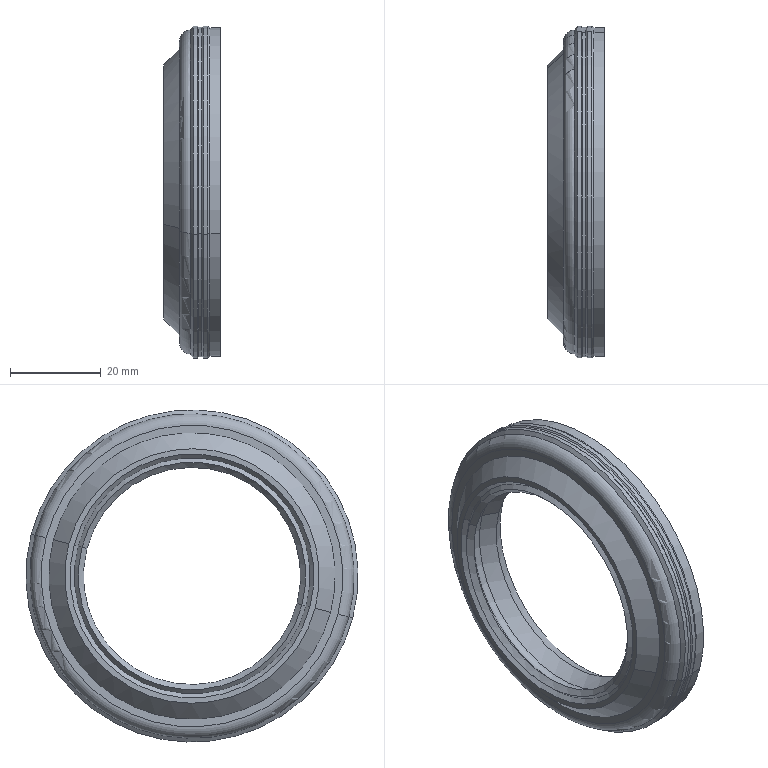Part | NX | features BREP 1 | 1 solid | 57 faces | box 12.5 x 73.025 x 73.025 mm | volume 15033 mm3 | cone 26 | torus 14 | cylinder 12 | plane 5 | commonest cylinder face diameters 53.4 x4 73.025 x4 72.34 x2 72.479 x2
STEP:
#1=CARTESIAN_POINT('',(-614.47,-25.827,-6.773));
#2=VERTEX_POINT('',#1);
#3=CARTESIAN_POINT('',(-614.47,25.827,6.773));
#4=VERTEX_POINT('',#3);
#5=CARTESIAN_POINT('',(-614.47,0.,0.));
#6=DIRECTION('',(-1.,0.,0.));
#7=DIRECTION('',(0.,-0.9673,-0.2537));
#8=AXIS2_PLACEMENT_3D('',#5,#6,#7);
#9=CIRCLE('',#8,26.7);
#10=EDGE_CURVE('',#2,#4,#9,.T.);
#11=ORIENTED_EDGE('',*,*,#10,.T.);
#12=CARTESIAN_POINT('',(-617.27,25.827,6.773));
#13=VERTEX_POINT('',#12);
#14=CARTESIAN_POINT('',(-615.87,25.827,6.773));
#15=DIRECTION('',(0.,-0.2537,0.9673));
#16=DIRECTION('',(0.,-0.9673,-0.2537));
#17=AXIS2_PLACEMENT_3D('',#14,#15,#16);
#18=CIRCLE('',#17,1.4);
#19=EDGE_CURVE('',#13,#4,#18,.F.);
#20=ORIENTED_EDGE('',*,*,#19,.F.);
#21=CARTESIAN_POINT('',(-617.27,-25.827,-6.773));
#22=VERTEX_POINT('',#21);
#23=CARTESIAN_POINT('',(-617.27,0.,0.));
#24=DIRECTION('',(1.,0.,0.));
#25=DIRECTION('',(0.,0.9673,0.2537));
#26=AXIS2_PLACEMENT_3D('',#23,#24,#25);
#27=CIRCLE('',#26,26.7);
#28=EDGE_CURVE('',#13,#22,#27,.T.);
#29=ORIENTED_EDGE('',*,*,#28,.T.);
#30=CARTESIAN_POINT('',(-615.87,-25.827,-6.773));
#31=DIRECTION('',(0.,0.2537,-0.9673));
#32=DIRECTION('',(0.,0.9673,0.2537));
#33=AXIS2_PLACEMENT_3D('',#30,#31,#32);
#34=CIRCLE('',#33,1.4);
#35=EDGE_CURVE('',#22,#2,#34,.F.);
#36=ORIENTED_EDGE('',*,*,#35,.T.);
#37=EDGE_LOOP('',(#11,#20,#29,#36));
#38=FACE_BOUND('',#37,.T.);
#39=CARTESIAN_POINT('',(-615.87,0.,0.));
#40=DIRECTION('',(-1.,0.,0.));
#41=DIRECTION('',(0.,0.9673,0.2537));
#42=AXIS2_PLACEMENT_3D('',#39,#40,#41);
#43=TOROIDAL_SURFACE('',#42,26.7,1.4);
#44=ADVANCED_FACE('',(#38),#43,.T.);
#45=CARTESIAN_POINT('',(-616.197,35.054,9.192));
#46=VERTEX_POINT('',#45);
#47=CARTESIAN_POINT('',(-616.197,-35.054,-9.192));
#48=VERTEX_POINT('',#47);
#49=CARTESIAN_POINT('',(-616.197,0.,0.));
#50=DIRECTION('',(1.,0.,0.));
#51=DIRECTION('',(0.,0.9673,0.2537));
#52=AXIS2_PLACEMENT_3D('',#49,#50,#51);
#53=CIRCLE('',#52,36.24);
#54=EDGE_CURVE('',#46,#48,#53,.T.);
#55=ORIENTED_EDGE('',*,*,#54,.T.);
#56=CARTESIAN_POINT('',(-615.494,-35.054,-9.192));
#57=VERTEX_POINT('',#56);
#58=CARTESIAN_POINT('',(-613.72,-35.054,-9.192));
#59=DIRECTION('',(1.,0.,0.));
#60=VECTOR('',#59,1000.);
#61=LINE('',#58,#60);
#62=EDGE_CURVE('',#48,#57,#61,.T.);
#63=ORIENTED_EDGE('',*,*,#62,.T.);
#64=CARTESIAN_POINT('',(-615.494,35.054,9.192));
#65=VERTEX_POINT('',#64);
#66=CARTESIAN_POINT('',(-615.494,0.,0.));
#67=DIRECTION('',(1.,0.,0.));
#68=DIRECTION('',(0.,0.9673,0.2537));
#69=AXIS2_PLACEMENT_3D('',#66,#67,#68);
#70=CIRCLE('',#69,36.24);
#71=EDGE_CURVE('',#65,#57,#70,.T.);
#72=ORIENTED_EDGE('',*,*,#71,.F.);
#73=CARTESIAN_POINT('',(-613.72,35.054,9.192));
#74=DIRECTION('',(1.,0.,0.));
#75=VECTOR('',#74,1000.);
#76=LINE('',#73,#75);
#77=EDGE_CURVE('',#46,#65,#76,.T.);
#78=ORIENTED_EDGE('',*,*,#77,.F.);
#79=EDGE_LOOP('',(#55,#63,#72,#78));
#80=FACE_BOUND('',#79,.T.);
#81=CARTESIAN_POINT('',(-613.72,0.,0.));
#82=DIRECTION('',(1.,0.,0.));
#83=DIRECTION('',(0.,-0.9673,-0.2537));
#84=AXIS2_PLACEMENT_3D('',#81,#82,#83);
#85=CYLINDRICAL_SURFACE('',#84,36.24);
#86=ADVANCED_FACE('',(#80),#85,.T.);
#87=ORIENTED_EDGE('',*,*,#71,.T.);
#88=CARTESIAN_POINT('',(-615.221,-35.318,-9.262));
#89=VERTEX_POINT('',#88);
#90=CARTESIAN_POINT('',(-615.221,-35.318,-9.262));
#91=DIRECTION('',(0.7071,-0.684,-0.1794));
#92=VECTOR('',#91,1000.);
#93=LINE('',#90,#92);
#94=EDGE_CURVE('',#57,#89,#93,.T.);
#95=ORIENTED_EDGE('',*,*,#94,.T.);
#96=CARTESIAN_POINT('',(-615.221,35.318,9.262));
#97=VERTEX_POINT('',#96);
#98=CARTESIAN_POINT('',(-615.221,0.,0.));
#99=DIRECTION('',(1.,0.,0.));
#100=DIRECTION('',(0.,0.9673,0.2537));
#101=AXIS2_PLACEMENT_3D('',#98,#99,#100);
#102=CIRCLE('',#101,36.513);
#103=EDGE_CURVE('',#97,#89,#102,.T.);
#104=ORIENTED_EDGE('',*,*,#103,.F.);
#105=CARTESIAN_POINT('',(-615.221,35.318,9.262));
#106=DIRECTION('',(0.7071,0.684,0.1794));
#107=VECTOR('',#106,1000.);
#108=LINE('',#105,#107);
#109=EDGE_CURVE('',#65,#97,#108,.T.);
#110=ORIENTED_EDGE('',*,*,#109,.F.);
#111=EDGE_LOOP('',(#87,#95,#104,#110));
#112=FACE_BOUND('',#111,.T.);
#113=CARTESIAN_POINT('',(-615.221,0.,0.));
#114=DIRECTION('',(1.,0.,0.));
#115=DIRECTION('',(0.,-0.9673,-0.2537));
#116=AXIS2_PLACEMENT_3D('',#113,#114,#115);
#117=CONICAL_SURFACE('',#116,36.513,0.7854);
#118=ADVANCED_FACE('',(#112),#117,.T.);
#119=ORIENTED_EDGE('',*,*,#103,.T.);
#120=CARTESIAN_POINT('',(-614.28,-35.318,-9.262));
#121=VERTEX_POINT('',#120);
#122=CARTESIAN_POINT('',(-613.72,-35.318,-9.262));
#123=DIRECTION('',(1.,0.,0.));
#124=VECTOR('',#123,1000.);
#125=LINE('',#122,#124);
#126=EDGE_CURVE('',#89,#121,#125,.T.);
#127=ORIENTED_EDGE('',*,*,#126,.T.);
#128=CARTESIAN_POINT('',(-614.28,35.318,9.262));
#129=VERTEX_POINT('',#128);
#130=CARTESIAN_POINT('',(-614.28,0.,0.));
#131=DIRECTION('',(1.,0.,0.));
#132=DIRECTION('',(0.,0.9673,0.2537));
#133=AXIS2_PLACEMENT_3D('',#130,#131,#132);
#134=CIRCLE('',#133,36.513);
#135=EDGE_CURVE('',#129,#121,#134,.T.);
#136=ORIENTED_EDGE('',*,*,#135,.F.);
#137=CARTESIAN_POINT('',(-613.72,35.318,9.262));
#138=DIRECTION('',(1.,0.,0.));
#139=VECTOR('',#138,1000.);
#140=LINE('',#137,#139);
#141=EDGE_CURVE('',#97,#129,#140,.T.);
#142=ORIENTED_EDGE('',*,*,#141,.F.);
#143=EDGE_LOOP('',(#119,#127,#136,#142));
#144=FACE_BOUND('',#143,.T.);
#145=CARTESIAN_POINT('',(-613.72,0.,0.));
#146=DIRECTION('',(1.,0.,0.));
#147=DIRECTION('',(0.,-0.9673,-0.2537));
#148=AXIS2_PLACEMENT_3D('',#145,#146,#147);
#149=CYLINDRICAL_SURFACE('',#148,36.513);
#150=ADVANCED_FACE('',(#144),#149,.T.);
#151=CARTESIAN_POINT('',(-613.72,-34.987,-9.175));
#152=VERTEX_POINT('',#151);
#153=CARTESIAN_POINT('',(-613.72,34.987,9.175));
#154=VERTEX_POINT('',#153);
#155=CARTESIAN_POINT('',(-613.72,0.,0.));
#156=DIRECTION('',(-1.,0.,0.));
#157=DIRECTION('',(0.,-0.9673,-0.2537));
#158=AXIS2_PLACEMENT_3D('',#155,#156,#157);
#159=CIRCLE('',#158,36.17);
#160=EDGE_CURVE('',#152,#154,#159,.T.);
#161=ORIENTED_EDGE('',*,*,#160,.T.);
#162=CARTESIAN_POINT('',(-613.72,34.987,9.175));
#163=DIRECTION('',(-0.8529,0.5049,0.1324));
#164=VECTOR('',#163,1000.);
#165=LINE('',#162,#164);
#166=EDGE_CURVE('',#129,#154,#165,.F.);
#167=ORIENTED_EDGE('',*,*,#166,.F.);
#168=ORIENTED_EDGE('',*,*,#135,.T.);
#169=CARTESIAN_POINT('',(-613.72,-34.987,-9.175));
#170=DIRECTION('',(-0.8529,-0.5049,-0.1324));
#171=VECTOR('',#170,1000.);
#172=LINE('',#169,#171);
#173=EDGE_CURVE('',#121,#152,#172,.F.);
#174=ORIENTED_EDGE('',*,*,#173,.T.);
#175=EDGE_LOOP('',(#161,#167,#168,#174));
#176=FACE_BOUND('',#175,.T.);
#177=CARTESIAN_POINT('',(-613.72,0.,0.));
#178=DIRECTION('',(-1.,0.,0.));
#179=DIRECTION('',(0.,0.9673,0.2537));
#180=AXIS2_PLACEMENT_3D('',#177,#178,#179);
#181=CONICAL_SURFACE('',#180,36.17,0.5492);
#182=ADVANCED_FACE('',(#176),#181,.T.);
#183=CARTESIAN_POINT('',(-618.051,34.481,9.042));
#184=VERTEX_POINT('',#183);
#185=CARTESIAN_POINT('',(-618.051,-34.481,-9.042));
#186=VERTEX_POINT('',#185);
#187=CARTESIAN_POINT('',(-618.051,0.,0.));
#188=DIRECTION('',(1.,0.,0.));
#189=DIRECTION('',(0.,0.9673,0.2537));
#190=AXIS2_PLACEMENT_3D('',#187,#188,#189);
#191=CIRCLE('',#190,35.647);
#192=EDGE_CURVE('',#184,#186,#191,.T.);
#193=ORIENTED_EDGE('',*,*,#192,.T.);
#194=CARTESIAN_POINT('',(-617.43,-35.318,-9.262));
#195=VERTEX_POINT('',#194);
#196=CARTESIAN_POINT('',(-617.43,-35.318,-9.262));
#197=DIRECTION('',(0.5827,-0.7861,-0.2061));
#198=VECTOR('',#197,1000.);
#199=LINE('',#196,#198);
#200=EDGE_CURVE('',#186,#195,#199,.T.);
#201=ORIENTED_EDGE('',*,*,#200,.T.);
#202=CARTESIAN_POINT('',(-617.43,35.318,9.262));
#203=VERTEX_POINT('',#202);
#204=CARTESIAN_POINT('',(-617.43,0.,0.));
#205=DIRECTION('',(1.,0.,0.));
#206=DIRECTION('',(0.,0.9673,0.2537));
#207=AXIS2_PLACEMENT_3D('',#204,#205,#206);
#208=CIRCLE('',#207,36.513);
#209=EDGE_CURVE('',#203,#195,#208,.T.);
#210=ORIENTED_EDGE('',*,*,#209,.F.);
#211=CARTESIAN_POINT('',(-617.43,35.318,9.262));
#212=DIRECTION('',(0.5827,0.7861,0.2061));
#213=VECTOR('',#212,1000.);
#214=LINE('',#211,#213);
#215=EDGE_CURVE('',#184,#203,#214,.T.);
#216=ORIENTED_EDGE('',*,*,#215,.F.);
#217=EDGE_LOOP('',(#193,#201,#210,#216));
#218=FACE_BOUND('',#217,.T.);
#219=CARTESIAN_POINT('',(-617.43,0.,0.));
#220=DIRECTION('',(1.,0.,0.));
#221=DIRECTION('',(0.,-0.9673,-0.2537));
#222=AXIS2_PLACEMENT_3D('',#219,#220,#221);
#223=CONICAL_SURFACE('',#222,36.513,0.9488);
#224=ADVANCED_FACE('',(#218),#223,.T.);
#225=ORIENTED_EDGE('',*,*,#209,.T.);
#226=CARTESIAN_POINT('',(-616.47,-35.318,-9.262));
#227=VERTEX_POINT('',#226);
#228=CARTESIAN_POINT('',(-613.72,-35.318,-9.262));
#229=DIRECTION('',(1.,0.,0.));
#230=VECTOR('',#229,1000.);
#231=LINE('',#228,#230);
#232=EDGE_CURVE('',#195,#227,#231,.T.);
#233=ORIENTED_EDGE('',*,*,#232,.T.);
#234=CARTESIAN_POINT('',(-616.47,35.318,9.262));
#235=VERTEX_POINT('',#234);
#236=CARTESIAN_POINT('',(-616.47,0.,0.));
#237=DIRECTION('',(1.,0.,0.));
#238=DIRECTION('',(0.,0.9673,0.2537));
#239=AXIS2_PLACEMENT_3D('',#236,#237,#238);
#240=CIRCLE('',#239,36.513);
#241=EDGE_CURVE('',#235,#227,#240,.T.);
#242=ORIENTED_EDGE('',*,*,#241,.F.);
#243=CARTESIAN_POINT('',(-613.72,35.318,9.262));
#244=DIRECTION('',(1.,0.,0.));
#245=VECTOR('',#244,1000.);
#246=LINE('',#243,#245);
#247=EDGE_CURVE('',#203,#235,#246,.T.);
#248=ORIENTED_EDGE('',*,*,#247,.F.);
#249=EDGE_LOOP('',(#225,#233,#242,#248));
#250=FACE_BOUND('',#249,.T.);
#251=CARTESIAN_POINT('',(-613.72,0.,0.));
#252=DIRECTION('',(1.,0.,0.));
#253=DIRECTION('',(0.,-0.9673,-0.2537));
#254=AXIS2_PLACEMENT_3D('',#251,#252,#253);
#255=CYLINDRICAL_SURFACE('',#254,36.513);
#256=ADVANCED_FACE('',(#250),#255,.T.);
#257=ORIENTED_EDGE('',*,*,#54,.F.);
#258=CARTESIAN_POINT('',(-616.197,35.054,9.192));
#259=DIRECTION('',(-0.7071,0.684,0.1794));
#260=VECTOR('',#259,1000.);
#261=LINE('',#258,#260);
#262=EDGE_CURVE('',#235,#46,#261,.F.);
#263=ORIENTED_EDGE('',*,*,#262,.F.);
#264=ORIENTED_EDGE('',*,*,#241,.T.);
#265=CARTESIAN_POINT('',(-616.197,-35.054,-9.192));
#266=DIRECTION('',(-0.7071,-0.684,-0.1794));
#267=VECTOR('',#266,1000.);
#268=LINE('',#265,#267);
#269=EDGE_CURVE('',#227,#48,#268,.F.);
#270=ORIENTED_EDGE('',*,*,#269,.T.);
#271=EDGE_LOOP('',(#257,#263,#264,#270));
#272=FACE_BOUND('',#271,.T.);
#273=CARTESIAN_POINT('',(-616.197,0.,0.));
#274=DIRECTION('',(-1.,0.,0.));
#275=DIRECTION('',(0.,0.9673,0.2537));
#276=AXIS2_PLACEMENT_3D('',#273,#274,#275);
#277=CONICAL_SURFACE('',#276,36.24,0.7854);
#278=ADVANCED_FACE('',(#272),#277,.T.);
#279=CARTESIAN_POINT('',(-611.42,-34.987,-9.175));
#280=VERTEX_POINT('',#279);
#281=CARTESIAN_POINT('',(-611.42,34.987,9.175));
#282=VERTEX_POINT('',#281);
#283=CARTESIAN_POINT('',(-611.42,0.,0.));
#284=DIRECTION('',(-1.,0.,0.));
#285=DIRECTION('',(0.,-0.9673,-0.2537));
#286=AXIS2_PLACEMENT_3D('',#283,#284,#285);
#287=CIRCLE('',#286,36.17);
#288=EDGE_CURVE('',#280,#282,#287,.T.);
#289=ORIENTED_EDGE('',*,*,#288,.T.);
#290=CARTESIAN_POINT('',(-623.62,34.987,9.175));
#291=DIRECTION('',(-1.,0.,0.));
#292=VECTOR('',#291,1000.);
#293=LINE('',#290,#292);
#294=EDGE_CURVE('',#154,#282,#293,.F.);
#295=ORIENTED_EDGE('',*,*,#294,.F.);
#296=ORIENTED_EDGE('',*,*,#160,.F.);
#297=CARTESIAN_POINT('',(-623.62,-34.987,-9.175));
#298=DIRECTION('',(-1.,0.,0.));
#299=VECTOR('',#298,1000.);
#300=LINE('',#297,#299);
#301=EDGE_CURVE('',#152,#280,#300,.F.);
#302=ORIENTED_EDGE('',*,*,#301,.T.);
#303=EDGE_LOOP('',(#289,#295,#296,#302));
#304=FACE_BOUND('',#303,.T.);
#305=CARTESIAN_POINT('',(-623.62,0.,0.));
#306=DIRECTION('',(-1.,0.,0.));
#307=DIRECTION('',(0.,0.9673,0.2537));
#308=AXIS2_PLACEMENT_3D('',#305,#306,#307);
#309=CYLINDRICAL_SURFACE('',#308,36.17);
#310=ADVANCED_FACE('',(#304),#309,.T.);
#311=ORIENTED_EDGE('',*,*,#192,.F.);
#312=CARTESIAN_POINT('',(-620.42,32.066,8.409));
#313=VERTEX_POINT('',#312);
#314=CARTESIAN_POINT('',(-617.92,32.066,8.409));
#315=DIRECTION('',(0.,-0.2537,0.9673));
#316=DIRECTION('',(0.,-0.9673,-0.2537));
#317=AXIS2_PLACEMENT_3D('',#314,#315,#316);
#318=CIRCLE('',#317,2.5);
#319=EDGE_CURVE('',#313,#184,#318,.F.);
#320=ORIENTED_EDGE('',*,*,#319,.F.);
#321=CARTESIAN_POINT('',(-620.42,-32.066,-8.409));
#322=VERTEX_POINT('',#321);
#323=CARTESIAN_POINT('',(-620.42,0.,0.));
#324=DIRECTION('',(-1.,0.,0.));
#325=DIRECTION('',(0.,-0.9673,-0.2537));
#326=AXIS2_PLACEMENT_3D('',#323,#324,#325);
#327=CIRCLE('',#326,33.15);
#328=EDGE_CURVE('',#322,#313,#327,.T.);
#329=ORIENTED_EDGE('',*,*,#328,.F.);
#330=CARTESIAN_POINT('',(-617.92,-32.066,-8.409));
#331=DIRECTION('',(0.,0.2537,-0.9673));
#332=DIRECTION('',(0.,0.9673,0.2537));
#333=AXIS2_PLACEMENT_3D('',#330,#331,#332);
#334=CIRCLE('',#333,2.5);
#335=EDGE_CURVE('',#322,#186,#334,.F.);
#336=ORIENTED_EDGE('',*,*,#335,.T.);
#337=EDGE_LOOP('',(#311,#320,#329,#336));
#338=FACE_BOUND('',#337,.T.);
#339=CARTESIAN_POINT('',(-617.92,0.,0.));
#340=DIRECTION('',(-1.,0.,0.));
#341=DIRECTION('',(0.,0.9673,0.2537));
#342=AXIS2_PLACEMENT_3D('',#339,#340,#341);
#343=TOROIDAL_SURFACE('',#342,33.15,2.5);
#344=ADVANCED_FACE('',(#338),#343,.T.);
#345=CARTESIAN_POINT('',(-615.87,23.094,6.056));
#346=VERTEX_POINT('',#345);
#347=CARTESIAN_POINT('',(-615.87,-23.094,-6.056));
#348=VERTEX_POINT('',#347);
#349=CARTESIAN_POINT('',(-615.87,0.,0.));
#350=DIRECTION('',(-1.,0.,0.));
#351=DIRECTION('',(0.,-0.9673,-0.2537));
#352=AXIS2_PLACEMENT_3D('',#349,#350,#351);
#353=CIRCLE('',#352,23.875);
#354=EDGE_CURVE('',#346,#348,#353,.T.);
#355=ORIENTED_EDGE('',*,*,#354,.F.);
#356=CARTESIAN_POINT('',(-619.575,24.542,6.436));
#357=VERTEX_POINT('',#356);
#358=CARTESIAN_POINT('',(-619.575,24.542,6.436));
#359=DIRECTION('',(-0.9272,0.3624,0.09502));
#360=VECTOR('',#359,1000.);
#361=LINE('',#358,#360);
#362=EDGE_CURVE('',#357,#346,#361,.F.);
#363=ORIENTED_EDGE('',*,*,#362,.F.);
#364=CARTESIAN_POINT('',(-619.575,-24.542,-6.436));
#365=VERTEX_POINT('',#364);
#366=CARTESIAN_POINT('',(-619.575,0.,0.));
#367=DIRECTION('',(-1.,0.,0.));
#368=DIRECTION('',(0.,-0.9673,-0.2537));
#369=AXIS2_PLACEMENT_3D('',#366,#367,#368);
#370=CIRCLE('',#369,25.372);
#371=EDGE_CURVE('',#357,#365,#370,.T.);
#372=ORIENTED_EDGE('',*,*,#371,.T.);
#373=CARTESIAN_POINT('',(-619.575,-24.542,-6.436));
#374=DIRECTION('',(-0.9272,-0.3624,-0.09502));
#375=VECTOR('',#374,1000.);
#376=LINE('',#373,#375);
#377=EDGE_CURVE('',#365,#348,#376,.F.);
#378=ORIENTED_EDGE('',*,*,#377,.T.);
#379=EDGE_LOOP('',(#355,#363,#372,#378));
#380=FACE_BOUND('',#379,.T.);
#381=CARTESIAN_POINT('',(-619.575,0.,0.));
#382=DIRECTION('',(-1.,0.,0.));
#383=DIRECTION('',(0.,0.9673,0.2537));
#384=AXIS2_PLACEMENT_3D('',#381,#382,#383);
#385=CONICAL_SURFACE('',#384,25.372,0.384);
#386=ADVANCED_FACE('',(#380),#385,.F.);
#387=ORIENTED_EDGE('',*,*,#354,.T.);
#388=CARTESIAN_POINT('',(-613.07,-24.666,-6.468));
#389=VERTEX_POINT('',#388);
#390=CARTESIAN_POINT('',(-615.87,-23.094,-6.056));
#391=DIRECTION('',(0.8649,-0.4855,-0.1273));
#392=VECTOR('',#391,1000.);
#393=LINE('',#390,#392);
#394=EDGE_CURVE('',#348,#389,#393,.T.);
#395=ORIENTED_EDGE('',*,*,#394,.T.);
#396=CARTESIAN_POINT('',(-613.07,24.666,6.468));
#397=VERTEX_POINT('',#396);
#398=CARTESIAN_POINT('',(-613.07,0.,0.));
#399=DIRECTION('',(-1.,0.,0.));
#400=DIRECTION('',(0.,-0.9673,-0.2537));
#401=AXIS2_PLACEMENT_3D('',#398,#399,#400);
#402=CIRCLE('',#401,25.5);
#403=EDGE_CURVE('',#397,#389,#402,.T.);
#404=ORIENTED_EDGE('',*,*,#403,.F.);
#405=CARTESIAN_POINT('',(-615.87,23.094,6.056));
#406=DIRECTION('',(0.8649,0.4855,0.1273));
#407=VECTOR('',#406,1000.);
#408=LINE('',#405,#407);
#409=EDGE_CURVE('',#346,#397,#408,.T.);
#410=ORIENTED_EDGE('',*,*,#409,.F.);
#411=EDGE_LOOP('',(#387,#395,#404,#410));
#412=FACE_BOUND('',#411,.T.);
#413=CARTESIAN_POINT('',(-615.87,0.,0.));
#414=DIRECTION('',(1.,0.,0.));
#415=DIRECTION('',(0.,-0.9673,-0.2537));
#416=AXIS2_PLACEMENT_3D('',#413,#414,#415);
#417=CONICAL_SURFACE('',#416,23.875,0.5259);
#418=ADVANCED_FACE('',(#412),#417,.F.);
#419=CARTESIAN_POINT('',(-613.07,-25.827,-6.773));
#420=VERTEX_POINT('',#419);
#421=CARTESIAN_POINT('',(-613.07,25.827,6.773));
#422=VERTEX_POINT('',#421);
#423=CARTESIAN_POINT('',(-613.07,0.,0.));
#424=DIRECTION('',(-1.,0.,0.));
#425=DIRECTION('',(0.,-0.9673,-0.2537));
#426=AXIS2_PLACEMENT_3D('',#423,#424,#425);
#427=CIRCLE('',#426,26.7);
#428=EDGE_CURVE('',#420,#422,#427,.T.);
#429=ORIENTED_EDGE('',*,*,#428,.T.);
#430=CARTESIAN_POINT('',(-623.92,25.827,6.773));
#431=DIRECTION('',(-1.,0.,0.));
#432=VECTOR('',#431,1000.);
#433=LINE('',#430,#432);
#434=EDGE_CURVE('',#4,#422,#433,.F.);
#435=ORIENTED_EDGE('',*,*,#434,.F.);
#436=ORIENTED_EDGE('',*,*,#10,.F.);
#437=CARTESIAN_POINT('',(-623.92,-25.827,-6.773));
#438=DIRECTION('',(-1.,0.,0.));
#439=VECTOR('',#438,1000.);
#440=LINE('',#437,#439);
#441=EDGE_CURVE('',#2,#420,#440,.F.);
#442=ORIENTED_EDGE('',*,*,#441,.T.);
#443=EDGE_LOOP('',(#429,#435,#436,#442));
#444=FACE_BOUND('',#443,.T.);
#445=CARTESIAN_POINT('',(-623.92,0.,0.));
#446=DIRECTION('',(-1.,0.,0.));
#447=DIRECTION('',(0.,0.9673,0.2537));
#448=AXIS2_PLACEMENT_3D('',#445,#446,#447);
#449=CYLINDRICAL_SURFACE('',#448,26.7);
#450=ADVANCED_FACE('',(#444),#449,.T.);
#451=ORIENTED_EDGE('',*,*,#28,.F.);
#452=CARTESIAN_POINT('',(-618.787,25.827,6.773));
#453=VERTEX_POINT('',#452);
#454=CARTESIAN_POINT('',(-623.92,25.827,6.773));
#455=DIRECTION('',(-1.,0.,0.));
#456=VECTOR('',#455,1000.);
#457=LINE('',#454,#456);
#458=EDGE_CURVE('',#453,#13,#457,.F.);
#459=ORIENTED_EDGE('',*,*,#458,.F.);
#460=CARTESIAN_POINT('',(-618.787,-25.827,-6.773));
#461=VERTEX_POINT('',#460);
#462=CARTESIAN_POINT('',(-618.787,0.,0.));
#463=DIRECTION('',(-1.,0.,0.));
#464=DIRECTION('',(0.,-0.9673,-0.2537));
#465=AXIS2_PLACEMENT_3D('',#462,#463,#464);
#466=CIRCLE('',#465,26.7);
#467=EDGE_CURVE('',#461,#453,#466,.T.);
#468=ORIENTED_EDGE('',*,*,#467,.F.);
#469=CARTESIAN_POINT('',(-623.92,-25.827,-6.773));
#470=DIRECTION('',(-1.,0.,0.));
#471=VECTOR('',#470,1000.);
#472=LINE('',#469,#471);
#473=EDGE_CURVE('',#461,#22,#472,.F.);
#474=ORIENTED_EDGE('',*,*,#473,.T.);
#475=EDGE_LOOP('',(#451,#459,#468,#474));
#476=FACE_BOUND('',#475,.T.);
#477=CARTESIAN_POINT('',(-623.92,0.,0.));
#478=DIRECTION('',(-1.,0.,0.));
#479=DIRECTION('',(0.,0.9673,0.2537));
#480=AXIS2_PLACEMENT_3D('',#477,#478,#479);
#481=CYLINDRICAL_SURFACE('',#480,26.7);
#482=ADVANCED_FACE('',(#476),#481,.T.);
#483=CARTESIAN_POINT('',(-619.07,26.487,6.946));
#484=VERTEX_POINT('',#483);
#485=CARTESIAN_POINT('',(-619.07,-26.487,-6.946));
#486=VERTEX_POINT('',#485);
#487=CARTESIAN_POINT('',(-619.07,0.,0.));
#488=DIRECTION('',(-1.,0.,0.));
#489=DIRECTION('',(0.,-0.9673,-0.2537));
#490=AXIS2_PLACEMENT_3D('',#487,#488,#489);
#491=CIRCLE('',#490,27.383);
#492=EDGE_CURVE('',#484,#486,#491,.T.);
#493=ORIENTED_EDGE('',*,*,#492,.F.);
#494=CARTESIAN_POINT('',(-618.787,26.214,6.874));
#495=DIRECTION('',(0.,-0.2537,0.9673));
#496=DIRECTION('',(0.,-0.9673,-0.2537));
#497=AXIS2_PLACEMENT_3D('',#494,#495,#496);
#498=CIRCLE('',#497,0.4);
#499=EDGE_CURVE('',#453,#484,#498,.F.);
#500=ORIENTED_EDGE('',*,*,#499,.F.);
#501=CARTESIAN_POINT('',(-618.787,0.,0.));
#502=DIRECTION('',(-1.,0.,0.));
#503=DIRECTION('',(0.,-0.9673,-0.2537));
#504=AXIS2_PLACEMENT_3D('',#501,#502,#503);
#505=CIRCLE('',#504,26.7);
#506=EDGE_CURVE('',#453,#461,#505,.T.);
#507=ORIENTED_EDGE('',*,*,#506,.T.);
#508=CARTESIAN_POINT('',(-618.787,-26.214,-6.874));
#509=DIRECTION('',(0.,0.2537,-0.9673));
#510=DIRECTION('',(0.,0.9673,0.2537));
#511=AXIS2_PLACEMENT_3D('',#508,#509,#510);
#512=CIRCLE('',#511,0.4);
#513=EDGE_CURVE('',#461,#486,#512,.F.);
#514=ORIENTED_EDGE('',*,*,#513,.T.);
#515=EDGE_LOOP('',(#493,#500,#507,#514));
#516=FACE_BOUND('',#515,.T.);
#517=CARTESIAN_POINT('',(-618.787,0.,0.));
#518=DIRECTION('',(-1.,0.,0.));
#519=DIRECTION('',(0.,0.9673,0.2537));
#520=AXIS2_PLACEMENT_3D('',#517,#518,#519);
#521=TOROIDAL_SURFACE('',#520,27.1,0.4);
#522=ADVANCED_FACE('',(#516),#521,.F.);
#523=ORIENTED_EDGE('',*,*,#492,.T.);
#524=CARTESIAN_POINT('',(-618.233,-27.297,-7.158));
#525=VERTEX_POINT('',#524);
#526=CARTESIAN_POINT('',(-619.07,-26.487,-6.946));
#527=DIRECTION('',(0.7071,-0.684,-0.1794));
#528=VECTOR('',#527,1000.);
#529=LINE('',#526,#528);
#530=EDGE_CURVE('',#486,#525,#529,.T.);
#531=ORIENTED_EDGE('',*,*,#530,.T.);
#532=CARTESIAN_POINT('',(-618.233,27.297,7.158));
#533=VERTEX_POINT('',#532);
#534=CARTESIAN_POINT('',(-618.233,0.,0.));
#535=DIRECTION('',(-1.,0.,0.));
#536=DIRECTION('',(0.,-0.9673,-0.2537));
#537=AXIS2_PLACEMENT_3D('',#534,#535,#536);
#538=CIRCLE('',#537,28.22);
#539=EDGE_CURVE('',#533,#525,#538,.T.);
#540=ORIENTED_EDGE('',*,*,#539,.F.);
#541=CARTESIAN_POINT('',(-619.07,26.487,6.946));
#542=DIRECTION('',(0.7071,0.684,0.1794));
#543=VECTOR('',#542,1000.);
#544=LINE('',#541,#543);
#545=EDGE_CURVE('',#484,#533,#544,.T.);
#546=ORIENTED_EDGE('',*,*,#545,.F.);
#547=EDGE_LOOP('',(#523,#531,#540,#546));
#548=FACE_BOUND('',#547,.T.);
#549=CARTESIAN_POINT('',(-619.07,0.,0.));
#550=DIRECTION('',(1.,0.,0.));
#551=DIRECTION('',(0.,-0.9673,-0.2537));
#552=AXIS2_PLACEMENT_3D('',#549,#550,#551);
#553=CONICAL_SURFACE('',#552,27.383,0.7854);
#554=ADVANCED_FACE('',(#548),#553,.F.);
#555=CARTESIAN_POINT('',(-618.233,0.,0.));
#556=DIRECTION('',(-1.,0.,0.));
#557=DIRECTION('',(0.,-0.9673,-0.2537));
#558=AXIS2_PLACEMENT_3D('',#555,#556,#557);
#559=CIRCLE('',#558,28.22);
#560=EDGE_CURVE('',#525,#533,#559,.T.);
#561=ORIENTED_EDGE('',*,*,#560,.T.);
#562=CARTESIAN_POINT('',(-617.12,29.896,7.84));
#563=VERTEX_POINT('',#562);
#564=CARTESIAN_POINT('',(-620.92,29.896,7.84));
#565=DIRECTION('',(0.,-0.2537,0.9673));
#566=DIRECTION('',(0.,-0.9673,-0.2537));
#567=AXIS2_PLACEMENT_3D('',#564,#565,#566);
#568=CIRCLE('',#567,3.8);
#569=EDGE_CURVE('',#563,#533,#568,.F.);
#570=ORIENTED_EDGE('',*,*,#569,.F.);
#571=CARTESIAN_POINT('',(-617.12,-29.896,-7.84));
#572=VERTEX_POINT('',#571);
#573=CARTESIAN_POINT('',(-617.12,0.,0.));
#574=DIRECTION('',(-1.,0.,0.));
#575=DIRECTION('',(0.,-0.9673,-0.2537));
#576=AXIS2_PLACEMENT_3D('',#573,#574,#575);
#577=CIRCLE('',#576,30.907);
#578=EDGE_CURVE('',#572,#563,#577,.T.);
#579=ORIENTED_EDGE('',*,*,#578,.F.);
#580=CARTESIAN_POINT('',(-620.92,-29.896,-7.84));
#581=DIRECTION('',(0.,0.2537,-0.9673));
#582=DIRECTION('',(0.,0.9673,0.2537));
#583=AXIS2_PLACEMENT_3D('',#580,#581,#582);
#584=CIRCLE('',#583,3.8);
#585=EDGE_CURVE('',#572,#525,#584,.F.);
#586=ORIENTED_EDGE('',*,*,#585,.T.);
#587=EDGE_LOOP('',(#561,#570,#579,#586));
#588=FACE_BOUND('',#587,.T.);
#589=CARTESIAN_POINT('',(-620.92,0.,0.));
#590=DIRECTION('',(-1.,0.,0.));
#591=DIRECTION('',(0.,0.9673,0.2537));
#592=AXIS2_PLACEMENT_3D('',#589,#590,#591);
#593=TOROIDAL_SURFACE('',#592,30.907,3.8);
#594=ADVANCED_FACE('',(#588),#593,.T.);
#595=CARTESIAN_POINT('',(-617.12,31.332,8.216));
#596=VERTEX_POINT('',#595);
#597=CARTESIAN_POINT('',(-617.12,-31.332,-8.216));
#598=VERTEX_POINT('',#597);
#599=CARTESIAN_POINT('',(-617.12,0.,0.));
#600=DIRECTION('',(-1.,0.,0.));
#601=DIRECTION('',(0.,-0.9673,-0.2537));
#602=AXIS2_PLACEMENT_3D('',#599,#600,#601);
#603=CIRCLE('',#602,32.391);
#604=EDGE_CURVE('',#596,#598,#603,.T.);
#605=ORIENTED_EDGE('',*,*,#604,.T.);
#606=CARTESIAN_POINT('',(-611.42,-31.62,-8.292));
#607=VERTEX_POINT('',#606);
#608=CARTESIAN_POINT('',(-617.12,-31.332,-8.216));
#609=DIRECTION('',(0.9986,-0.05062,-0.01328));
#610=VECTOR('',#609,1000.);
#611=LINE('',#608,#610);
#612=EDGE_CURVE('',#598,#607,#611,.T.);
#613=ORIENTED_EDGE('',*,*,#612,.T.);
#614=CARTESIAN_POINT('',(-611.42,31.62,8.292));
#615=VERTEX_POINT('',#614);
#616=CARTESIAN_POINT('',(-611.42,0.,0.));
#617=DIRECTION('',(-1.,0.,0.));
#618=DIRECTION('',(0.,-0.9673,-0.2537));
#619=AXIS2_PLACEMENT_3D('',#616,#617,#618);
#620=CIRCLE('',#619,32.69);
#621=EDGE_CURVE('',#615,#607,#620,.T.);
#622=ORIENTED_EDGE('',*,*,#621,.F.);
#623=CARTESIAN_POINT('',(-617.12,31.332,8.216));
#624=DIRECTION('',(0.9986,0.05062,0.01328));
#625=VECTOR('',#624,1000.);
#626=LINE('',#623,#625);
#627=EDGE_CURVE('',#596,#615,#626,.T.);
#628=ORIENTED_EDGE('',*,*,#627,.F.);
#629=EDGE_LOOP('',(#605,#613,#622,#628));
#630=FACE_BOUND('',#629,.T.);
#631=CARTESIAN_POINT('',(-617.12,0.,0.));
#632=DIRECTION('',(1.,0.,0.));
#633=DIRECTION('',(0.,-0.9673,-0.2537));
#634=AXIS2_PLACEMENT_3D('',#631,#632,#633);
#635=CONICAL_SURFACE('',#634,32.391,0.05236);
#636=ADVANCED_FACE('',(#630),#635,.F.);
#637=CARTESIAN_POINT('',(-623.92,-27.063,-7.097));
#638=VERTEX_POINT('',#637);
#639=CARTESIAN_POINT('',(-623.92,27.063,7.097));
#640=VERTEX_POINT('',#639);
#641=CARTESIAN_POINT('',(-623.92,0.,0.));
#642=DIRECTION('',(-1.,0.,0.));
#643=DIRECTION('',(0.,-0.9673,-0.2537));
#644=AXIS2_PLACEMENT_3D('',#641,#642,#643);
#645=CIRCLE('',#644,27.978);
#646=EDGE_CURVE('',#638,#640,#645,.T.);
#647=ORIENTED_EDGE('',*,*,#646,.F.);
#648=CARTESIAN_POINT('',(-620.42,-30.448,-7.984));
#649=VERTEX_POINT('',#648);
#650=CARTESIAN_POINT('',(-620.42,-30.448,-7.984));
#651=DIRECTION('',(0.7071,-0.684,-0.1794));
#652=VECTOR('',#651,1000.);
#653=LINE('',#650,#652);
#654=EDGE_CURVE('',#638,#649,#653,.T.);
#655=ORIENTED_EDGE('',*,*,#654,.T.);
#656=CARTESIAN_POINT('',(-620.42,30.448,7.984));
#657=VERTEX_POINT('',#656);
#658=CARTESIAN_POINT('',(-620.42,0.,0.));
#659=DIRECTION('',(-1.,0.,0.));
#660=DIRECTION('',(0.,0.9673,0.2537));
#661=AXIS2_PLACEMENT_3D('',#658,#659,#660);
#662=CIRCLE('',#661,31.478);
#663=EDGE_CURVE('',#649,#657,#662,.T.);
#664=ORIENTED_EDGE('',*,*,#663,.T.);
#665=CARTESIAN_POINT('',(-620.42,30.448,7.984));
#666=DIRECTION('',(0.7071,0.684,0.1794));
#667=VECTOR('',#666,1000.);
#668=LINE('',#665,#667);
#669=EDGE_CURVE('',#640,#657,#668,.T.);
#670=ORIENTED_EDGE('',*,*,#669,.F.);
#671=EDGE_LOOP('',(#647,#655,#664,#670));
#672=FACE_BOUND('',#671,.T.);
#673=CARTESIAN_POINT('',(-620.42,0.,0.));
#674=DIRECTION('',(1.,0.,0.));
#675=DIRECTION('',(0.,-0.9673,-0.2537));
#676=AXIS2_PLACEMENT_3D('',#673,#674,#675);
#677=CONICAL_SURFACE('',#676,31.478,0.7854);
#678=ADVANCED_FACE('',(#672),#677,.T.);
#679=CARTESIAN_POINT('',(-623.015,25.058,6.571));
#680=VERTEX_POINT('',#679);
#681=CARTESIAN_POINT('',(-623.015,-25.058,-6.571));
#682=VERTEX_POINT('',#681);
#683=CARTESIAN_POINT('',(-623.015,0.,0.));
#684=DIRECTION('',(-1.,0.,0.));
#685=DIRECTION('',(0.,-0.9673,-0.2537));
#686=AXIS2_PLACEMENT_3D('',#683,#684,#685);
#687=CIRCLE('',#686,25.905);
#688=EDGE_CURVE('',#680,#682,#687,.T.);
#689=ORIENTED_EDGE('',*,*,#688,.F.);
#690=CARTESIAN_POINT('',(-623.92,25.933,6.8));
#691=VERTEX_POINT('',#690);
#692=CARTESIAN_POINT('',(-623.92,25.933,6.8));
#693=DIRECTION('',(-0.7071,0.684,0.1794));
#694=VECTOR('',#693,1000.);
#695=LINE('',#692,#694);
#696=EDGE_CURVE('',#691,#680,#695,.F.);
#697=ORIENTED_EDGE('',*,*,#696,.F.);
#698=CARTESIAN_POINT('',(-623.92,-25.933,-6.8));
#699=VERTEX_POINT('',#698);
#700=CARTESIAN_POINT('',(-623.92,0.,0.));
#701=DIRECTION('',(-1.,0.,0.));
#702=DIRECTION('',(0.,-0.9673,-0.2537));
#703=AXIS2_PLACEMENT_3D('',#700,#701,#702);
#704=CIRCLE('',#703,26.81);
#705=EDGE_CURVE('',#691,#699,#704,.T.);
#706=ORIENTED_EDGE('',*,*,#705,.T.);
#707=CARTESIAN_POINT('',(-623.92,-25.933,-6.8));
#708=DIRECTION('',(-0.7071,-0.684,-0.1794));
#709=VECTOR('',#708,1000.);
#710=LINE('',#707,#709);
#711=EDGE_CURVE('',#699,#682,#710,.F.);
#712=ORIENTED_EDGE('',*,*,#711,.T.);
#713=EDGE_LOOP('',(#689,#697,#706,#712));
#714=FACE_BOUND('',#713,.T.);
#715=CARTESIAN_POINT('',(-623.92,0.,0.));
#716=DIRECTION('',(-1.,0.,0.));
#717=DIRECTION('',(0.,0.9673,0.2537));
#718=AXIS2_PLACEMENT_3D('',#715,#716,#717);
#719=CONICAL_SURFACE('',#718,26.81,0.7854);
#720=ADVANCED_FACE('',(#714),#719,.F.);
#721=CARTESIAN_POINT('',(-623.92,-24.182,-6.341));
#722=VERTEX_POINT('',#721);
#723=CARTESIAN_POINT('',(-623.92,24.182,6.341));
#724=VERTEX_POINT('',#723);
#725=CARTESIAN_POINT('',(-623.92,0.,0.));
#726=DIRECTION('',(-1.,0.,0.));
#727=DIRECTION('',(0.,-0.9673,-0.2537));
#728=AXIS2_PLACEMENT_3D('',#725,#726,#727);
#729=CIRCLE('',#728,25.);
#730=EDGE_CURVE('',#722,#724,#729,.T.);
#731=ORIENTED_EDGE('',*,*,#730,.F.);
#732=CARTESIAN_POINT('',(-623.015,-25.058,-6.571));
#733=DIRECTION('',(0.7071,-0.684,-0.1794));
#734=VECTOR('',#733,1000.);
#735=LINE('',#732,#734);
#736=EDGE_CURVE('',#722,#682,#735,.T.);
#737=ORIENTED_EDGE('',*,*,#736,.T.);
#738=CARTESIAN_POINT('',(-623.015,0.,0.));
#739=DIRECTION('',(-1.,0.,0.));
#740=DIRECTION('',(0.,-0.9673,-0.2537));
#741=AXIS2_PLACEMENT_3D('',#738,#739,#740);
#742=CIRCLE('',#741,25.905);
#743=EDGE_CURVE('',#682,#680,#742,.T.);
#744=ORIENTED_EDGE('',*,*,#743,.T.);
#745=CARTESIAN_POINT('',(-623.015,25.058,6.571));
#746=DIRECTION('',(0.7071,0.684,0.1794));
#747=VECTOR('',#746,1000.);
#748=LINE('',#745,#747);
#749=EDGE_CURVE('',#724,#680,#748,.T.);
#750=ORIENTED_EDGE('',*,*,#749,.F.);
#751=EDGE_LOOP('',(#731,#737,#744,#750));
#752=FACE_BOUND('',#751,.T.);
#753=CARTESIAN_POINT('',(-623.015,0.,0.));
#754=DIRECTION('',(1.,0.,0.));
#755=DIRECTION('',(0.,-0.9673,-0.2537));
#756=AXIS2_PLACEMENT_3D('',#753,#754,#755);
#757=CONICAL_SURFACE('',#756,25.905,0.7854);
#758=ADVANCED_FACE('',(#752),#757,.T.);
#759=CARTESIAN_POINT('',(-622.795,23.094,6.056));
#760=VERTEX_POINT('',#759);
#761=CARTESIAN_POINT('',(-622.795,-23.094,-6.056));
#762=VERTEX_POINT('',#761);
#763=CARTESIAN_POINT('',(-622.795,0.,0.));
#764=DIRECTION('',(-1.,0.,0.));
#765=DIRECTION('',(0.,-0.9673,-0.2537));
#766=AXIS2_PLACEMENT_3D('',#763,#764,#765);
#767=CIRCLE('',#766,23.875);
#768=EDGE_CURVE('',#760,#762,#767,.T.);
#769=ORIENTED_EDGE('',*,*,#768,.F.);
#770=CARTESIAN_POINT('',(-623.92,24.182,6.341));
#771=DIRECTION('',(-0.7071,0.684,0.1794));
#772=VECTOR('',#771,1000.);
#773=LINE('',#770,#772);
#774=EDGE_CURVE('',#724,#760,#773,.F.);
#775=ORIENTED_EDGE('',*,*,#774,.F.);
#776=CARTESIAN_POINT('',(-623.92,0.,0.));
#777=DIRECTION('',(-1.,0.,0.));
#778=DIRECTION('',(0.,-0.9673,-0.2537));
#779=AXIS2_PLACEMENT_3D('',#776,#777,#778);
#780=CIRCLE('',#779,25.);
#781=EDGE_CURVE('',#724,#722,#780,.T.);
#782=ORIENTED_EDGE('',*,*,#781,.T.);
#783=CARTESIAN_POINT('',(-623.92,-24.182,-6.341));
#784=DIRECTION('',(-0.7071,-0.684,-0.1794));
#785=VECTOR('',#784,1000.);
#786=LINE('',#783,#785);
#787=EDGE_CURVE('',#722,#762,#786,.F.);
#788=ORIENTED_EDGE('',*,*,#787,.T.);
#789=EDGE_LOOP('',(#769,#775,#782,#788));
#790=FACE_BOUND('',#789,.T.);
#791=CARTESIAN_POINT('',(-623.92,0.,0.));
#792=DIRECTION('',(-1.,0.,0.));
#793=DIRECTION('',(0.,0.9673,0.2537));
#794=AXIS2_PLACEMENT_3D('',#791,#792,#793);
#795=CONICAL_SURFACE('',#794,25.,0.7854);
#796=ADVANCED_FACE('',(#790),#795,.F.);
#797=ORIENTED_EDGE('',*,*,#768,.T.);
#798=CARTESIAN_POINT('',(-621.738,-24.116,-6.324));
#799=VERTEX_POINT('',#798);
#800=CARTESIAN_POINT('',(-622.795,-23.094,-6.056));
#801=DIRECTION('',(0.7071,-0.684,-0.1794));
#802=VECTOR('',#801,1000.);
#803=LINE('',#800,#802);
#804=EDGE_CURVE('',#762,#799,#803,.T.);
#805=ORIENTED_EDGE('',*,*,#804,.T.);
#806=CARTESIAN_POINT('',(-621.738,24.116,6.324));
#807=VERTEX_POINT('',#806);
#808=CARTESIAN_POINT('',(-621.738,0.,0.));
#809=DIRECTION('',(-1.,0.,0.));
#810=DIRECTION('',(0.,-0.9673,-0.2537));
#811=AXIS2_PLACEMENT_3D('',#808,#809,#810);
#812=CIRCLE('',#811,24.932);
#813=EDGE_CURVE('',#807,#799,#812,.T.);
#814=ORIENTED_EDGE('',*,*,#813,.F.);
#815=CARTESIAN_POINT('',(-622.795,23.094,6.056));
#816=DIRECTION('',(0.7071,0.684,0.1794));
#817=VECTOR('',#816,1000.);
#818=LINE('',#815,#817);
#819=EDGE_CURVE('',#760,#807,#818,.T.);
#820=ORIENTED_EDGE('',*,*,#819,.F.);
#821=EDGE_LOOP('',(#797,#805,#814,#820));
#822=FACE_BOUND('',#821,.T.);
#823=CARTESIAN_POINT('',(-622.795,0.,0.));
#824=DIRECTION('',(1.,0.,0.));
#825=DIRECTION('',(0.,-0.9673,-0.2537));
#826=AXIS2_PLACEMENT_3D('',#823,#824,#825);
#827=CONICAL_SURFACE('',#826,23.875,0.7854);
#828=ADVANCED_FACE('',(#822),#827,.F.);
#829=ORIENTED_EDGE('',*,*,#371,.F.);
#830=CARTESIAN_POINT('',(-620.324,22.748,5.965));
#831=DIRECTION('',(0.,-0.2537,0.9673));
#832=DIRECTION('',(0.,-0.9673,-0.2537));
#833=AXIS2_PLACEMENT_3D('',#830,#831,#832);
#834=CIRCLE('',#833,2.);
#835=EDGE_CURVE('',#807,#357,#834,.F.);
#836=ORIENTED_EDGE('',*,*,#835,.F.);
#837=ORIENTED_EDGE('',*,*,#813,.T.);
#838=CARTESIAN_POINT('',(-620.324,-22.748,-5.965));
#839=DIRECTION('',(0.,0.2537,-0.9673));
#840=DIRECTION('',(0.,0.9673,0.2537));
#841=AXIS2_PLACEMENT_3D('',#838,#839,#840);
#842=CIRCLE('',#841,2.);
#843=EDGE_CURVE('',#799,#365,#842,.F.);
#844=ORIENTED_EDGE('',*,*,#843,.T.);
#845=EDGE_LOOP('',(#829,#836,#837,#844));
#846=FACE_BOUND('',#845,.T.);
#847=CARTESIAN_POINT('',(-620.324,0.,0.));
#848=DIRECTION('',(-1.,0.,0.));
#849=DIRECTION('',(0.,0.9673,0.2537));
#850=AXIS2_PLACEMENT_3D('',#847,#848,#849);
#851=TOROIDAL_SURFACE('',#850,23.517,2.);
#852=ADVANCED_FACE('',(#846),#851,.F.);
#853=ORIENTED_EDGE('',*,*,#835,.T.);
#854=CARTESIAN_POINT('',(-619.575,0.,0.));
#855=DIRECTION('',(-1.,0.,0.));
#856=DIRECTION('',(0.,-0.9673,-0.2537));
#857=AXIS2_PLACEMENT_3D('',#854,#855,#856);
#858=CIRCLE('',#857,25.372);
#859=EDGE_CURVE('',#365,#357,#858,.T.);
#860=ORIENTED_EDGE('',*,*,#859,.F.);
#861=ORIENTED_EDGE('',*,*,#843,.F.);
#862=CARTESIAN_POINT('',(-621.738,0.,0.));
#863=DIRECTION('',(-1.,0.,0.));
#864=DIRECTION('',(0.,-0.9673,-0.2537));
#865=AXIS2_PLACEMENT_3D('',#862,#863,#864);
#866=CIRCLE('',#865,24.932);
#867=EDGE_CURVE('',#799,#807,#866,.T.);
#868=ORIENTED_EDGE('',*,*,#867,.T.);
#869=EDGE_LOOP('',(#853,#860,#861,#868));
#870=FACE_BOUND('',#869,.T.);
#871=CARTESIAN_POINT('',(-620.324,0.,0.));
#872=DIRECTION('',(-1.,0.,0.));
#873=DIRECTION('',(0.,0.9673,0.2537));
#874=AXIS2_PLACEMENT_3D('',#871,#872,#873);
#875=TOROIDAL_SURFACE('',#874,23.517,2.);
#876=ADVANCED_FACE('',(#870),#875,.F.);
#877=ORIENTED_EDGE('',*,*,#804,.F.);
#878=CARTESIAN_POINT('',(-622.795,0.,0.));
#879=DIRECTION('',(-1.,0.,0.));
#880=DIRECTION('',(0.,-0.9673,-0.2537));
#881=AXIS2_PLACEMENT_3D('',#878,#879,#880);
#882=CIRCLE('',#881,23.875);
#883=EDGE_CURVE('',#762,#760,#882,.T.);
#884=ORIENTED_EDGE('',*,*,#883,.T.);
#885=ORIENTED_EDGE('',*,*,#819,.T.);
#886=ORIENTED_EDGE('',*,*,#867,.F.);
#887=EDGE_LOOP('',(#877,#884,#885,#886));
#888=FACE_BOUND('',#887,.T.);
#889=CARTESIAN_POINT('',(-622.795,0.,0.));
#890=DIRECTION('',(1.,0.,0.));
#891=DIRECTION('',(0.,-0.9673,-0.2537));
#892=AXIS2_PLACEMENT_3D('',#889,#890,#891);
#893=CONICAL_SURFACE('',#892,23.875,0.7854);
#894=ADVANCED_FACE('',(#888),#893,.F.);
#895=ORIENTED_EDGE('',*,*,#774,.T.);
#896=ORIENTED_EDGE('',*,*,#883,.F.);
#897=ORIENTED_EDGE('',*,*,#787,.F.);
#898=ORIENTED_EDGE('',*,*,#730,.T.);
#899=EDGE_LOOP('',(#895,#896,#897,#898));
#900=FACE_BOUND('',#899,.T.);
#901=CARTESIAN_POINT('',(-623.92,0.,0.));
#902=DIRECTION('',(-1.,0.,0.));
#903=DIRECTION('',(0.,0.9673,0.2537));
#904=AXIS2_PLACEMENT_3D('',#901,#902,#903);
#905=CONICAL_SURFACE('',#904,25.,0.7854);
#906=ADVANCED_FACE('',(#900),#905,.F.);
#907=ORIENTED_EDGE('',*,*,#736,.F.);
#908=ORIENTED_EDGE('',*,*,#781,.F.);
#909=ORIENTED_EDGE('',*,*,#749,.T.);
#910=ORIENTED_EDGE('',*,*,#688,.T.);
#911=EDGE_LOOP('',(#907,#908,#909,#910));
#912=FACE_BOUND('',#911,.T.);
#913=CARTESIAN_POINT('',(-623.015,0.,0.));
#914=DIRECTION('',(1.,0.,0.));
#915=DIRECTION('',(0.,-0.9673,-0.2537));
#916=AXIS2_PLACEMENT_3D('',#913,#914,#915);
#917=CONICAL_SURFACE('',#916,25.905,0.7854);
#918=ADVANCED_FACE('',(#912),#917,.T.);
#919=ORIENTED_EDGE('',*,*,#696,.T.);
#920=ORIENTED_EDGE('',*,*,#743,.F.);
#921=ORIENTED_EDGE('',*,*,#711,.F.);
#922=CARTESIAN_POINT('',(-623.92,0.,0.));
#923=DIRECTION('',(-1.,0.,0.));
#924=DIRECTION('',(0.,-0.9673,-0.2537));
#925=AXIS2_PLACEMENT_3D('',#922,#923,#924);
#926=CIRCLE('',#925,26.81);
#927=EDGE_CURVE('',#699,#691,#926,.T.);
#928=ORIENTED_EDGE('',*,*,#927,.T.);
#929=EDGE_LOOP('',(#919,#920,#921,#928));
#930=FACE_BOUND('',#929,.T.);
#931=CARTESIAN_POINT('',(-623.92,0.,0.));
#932=DIRECTION('',(-1.,0.,0.));
#933=DIRECTION('',(0.,0.9673,0.2537));
#934=AXIS2_PLACEMENT_3D('',#931,#932,#933);
#935=CONICAL_SURFACE('',#934,26.81,0.7854);
#936=ADVANCED_FACE('',(#930),#935,.F.);
#937=ORIENTED_EDGE('',*,*,#927,.F.);
#938=ORIENTED_EDGE('',*,*,#705,.F.);
#939=EDGE_LOOP('',(#937,#938));
#940=FACE_BOUND('',#939,.T.);
#941=CARTESIAN_POINT('',(-623.92,0.,0.));
#942=DIRECTION('',(-1.,0.,0.));
#943=DIRECTION('',(0.,-0.9673,-0.2537));
#944=AXIS2_PLACEMENT_3D('',#941,#942,#943);
#945=CIRCLE('',#944,27.978);
#946=EDGE_CURVE('',#640,#638,#945,.T.);
#947=ORIENTED_EDGE('',*,*,#946,.T.);
#948=ORIENTED_EDGE('',*,*,#646,.T.);
#949=EDGE_LOOP('',(#947,#948));
#950=FACE_BOUND('',#949,.T.);
#951=CARTESIAN_POINT('',(-623.92,-7.097,27.063));
#952=DIRECTION('',(1.,0.,0.));
#953=DIRECTION('',(0.,-0.9673,-0.2537));
#954=AXIS2_PLACEMENT_3D('',#951,#952,#953);
#955=PLANE('',#954);
#956=ADVANCED_FACE('',(#940,#950),#955,.F.);
#957=ORIENTED_EDGE('',*,*,#654,.F.);
#958=ORIENTED_EDGE('',*,*,#946,.F.);
#959=ORIENTED_EDGE('',*,*,#669,.T.);
#960=CARTESIAN_POINT('',(-620.42,0.,0.));
#961=DIRECTION('',(-1.,0.,0.));
#962=DIRECTION('',(0.,0.9673,0.2537));
#963=AXIS2_PLACEMENT_3D('',#960,#961,#962);
#964=CIRCLE('',#963,31.478);
#965=EDGE_CURVE('',#657,#649,#964,.T.);
#966=ORIENTED_EDGE('',*,*,#965,.T.);
#967=EDGE_LOOP('',(#957,#958,#959,#966));
#968=FACE_BOUND('',#967,.T.);
#969=CARTESIAN_POINT('',(-620.42,0.,0.));
#970=DIRECTION('',(1.,0.,0.));
#971=DIRECTION('',(0.,-0.9673,-0.2537));
#972=AXIS2_PLACEMENT_3D('',#969,#970,#971);
#973=CONICAL_SURFACE('',#972,31.478,0.7854);
#974=ADVANCED_FACE('',(#968),#973,.T.);
#975=ORIENTED_EDGE('',*,*,#612,.F.);
#976=CARTESIAN_POINT('',(-617.12,0.,0.));
#977=DIRECTION('',(-1.,0.,0.));
#978=DIRECTION('',(0.,-0.9673,-0.2537));
#979=AXIS2_PLACEMENT_3D('',#976,#977,#978);
#980=CIRCLE('',#979,32.391);
#981=EDGE_CURVE('',#598,#596,#980,.T.);
#982=ORIENTED_EDGE('',*,*,#981,.T.);
#983=ORIENTED_EDGE('',*,*,#627,.T.);
#984=CARTESIAN_POINT('',(-611.42,0.,0.));
#985=DIRECTION('',(-1.,0.,0.));
#986=DIRECTION('',(0.,-0.9673,-0.2537));
#987=AXIS2_PLACEMENT_3D('',#984,#985,#986);
#988=CIRCLE('',#987,32.69);
#989=EDGE_CURVE('',#607,#615,#988,.T.);
#990=ORIENTED_EDGE('',*,*,#989,.F.);
#991=EDGE_LOOP('',(#975,#982,#983,#990));
#992=FACE_BOUND('',#991,.T.);
#993=CARTESIAN_POINT('',(-617.12,0.,0.));
#994=DIRECTION('',(1.,0.,0.));
#995=DIRECTION('',(0.,-0.9673,-0.2537));
#996=AXIS2_PLACEMENT_3D('',#993,#994,#995);
#997=CONICAL_SURFACE('',#996,32.391,0.05236);
#998=ADVANCED_FACE('',(#992),#997,.F.);
#999=ORIENTED_EDGE('',*,*,#604,.F.);
#1000=ORIENTED_EDGE('',*,*,#981,.F.);
#1001=EDGE_LOOP('',(#999,#1000));
#1002=FACE_BOUND('',#1001,.T.);
#1003=ORIENTED_EDGE('',*,*,#578,.T.);
#1004=CARTESIAN_POINT('',(-617.12,0.,0.));
#1005=DIRECTION('',(-1.,0.,0.));
#1006=DIRECTION('',(0.,-0.9673,-0.2537));
#1007=AXIS2_PLACEMENT_3D('',#1004,#1005,#1006);
#1008=CIRCLE('',#1007,30.907);
#1009=EDGE_CURVE('',#563,#572,#1008,.T.);
#1010=ORIENTED_EDGE('',*,*,#1009,.T.);
#1011=EDGE_LOOP('',(#1003,#1010));
#1012=FACE_BOUND('',#1011,.T.);
#1013=CARTESIAN_POINT('',(-617.12,-7.84,29.896));
#1014=DIRECTION('',(-1.,0.,0.));
#1015=DIRECTION('',(0.,0.9673,0.2537));
#1016=AXIS2_PLACEMENT_3D('',#1013,#1014,#1015);
#1017=PLANE('',#1016);
#1018=ADVANCED_FACE('',(#1002,#1012),#1017,.F.);
#1019=ORIENTED_EDGE('',*,*,#569,.T.);
#1020=ORIENTED_EDGE('',*,*,#539,.T.);
#1021=ORIENTED_EDGE('',*,*,#585,.F.);
#1022=ORIENTED_EDGE('',*,*,#1009,.F.);
#1023=EDGE_LOOP('',(#1019,#1020,#1021,#1022));
#1024=FACE_BOUND('',#1023,.T.);
#1025=CARTESIAN_POINT('',(-620.92,0.,0.));
#1026=DIRECTION('',(-1.,0.,0.));
#1027=DIRECTION('',(0.,0.9673,0.2537));
#1028=AXIS2_PLACEMENT_3D('',#1025,#1026,#1027);
#1029=TOROIDAL_SURFACE('',#1028,30.907,3.8);
#1030=ADVANCED_FACE('',(#1024),#1029,.T.);
#1031=ORIENTED_EDGE('',*,*,#530,.F.);
#1032=CARTESIAN_POINT('',(-619.07,0.,0.));
#1033=DIRECTION('',(-1.,0.,0.));
#1034=DIRECTION('',(0.,-0.9673,-0.2537));
#1035=AXIS2_PLACEMENT_3D('',#1032,#1033,#1034);
#1036=CIRCLE('',#1035,27.383);
#1037=EDGE_CURVE('',#486,#484,#1036,.T.);
#1038=ORIENTED_EDGE('',*,*,#1037,.T.);
#1039=ORIENTED_EDGE('',*,*,#545,.T.);
#1040=ORIENTED_EDGE('',*,*,#560,.F.);
#1041=EDGE_LOOP('',(#1031,#1038,#1039,#1040));
#1042=FACE_BOUND('',#1041,.T.);
#1043=CARTESIAN_POINT('',(-619.07,0.,0.));
#1044=DIRECTION('',(1.,0.,0.));
#1045=DIRECTION('',(0.,-0.9673,-0.2537));
#1046=AXIS2_PLACEMENT_3D('',#1043,#1044,#1045);
#1047=CONICAL_SURFACE('',#1046,27.383,0.7854);
#1048=ADVANCED_FACE('',(#1042),#1047,.F.);
#1049=ORIENTED_EDGE('',*,*,#499,.T.);
#1050=ORIENTED_EDGE('',*,*,#1037,.F.);
#1051=ORIENTED_EDGE('',*,*,#513,.F.);
#1052=ORIENTED_EDGE('',*,*,#467,.T.);
#1053=EDGE_LOOP('',(#1049,#1050,#1051,#1052));
#1054=FACE_BOUND('',#1053,.T.);
#1055=CARTESIAN_POINT('',(-618.787,0.,0.));
#1056=DIRECTION('',(-1.,0.,0.));
#1057=DIRECTION('',(0.,0.9673,0.2537));
#1058=AXIS2_PLACEMENT_3D('',#1055,#1056,#1057);
#1059=TOROIDAL_SURFACE('',#1058,27.1,0.4);
#1060=ADVANCED_FACE('',(#1054),#1059,.F.);
#1061=ORIENTED_EDGE('',*,*,#458,.T.);
#1062=CARTESIAN_POINT('',(-617.27,0.,0.));
#1063=DIRECTION('',(1.,0.,0.));
#1064=DIRECTION('',(0.,0.9673,0.2537));
#1065=AXIS2_PLACEMENT_3D('',#1062,#1063,#1064);
#1066=CIRCLE('',#1065,26.7);
#1067=EDGE_CURVE('',#22,#13,#1066,.T.);
#1068=ORIENTED_EDGE('',*,*,#1067,.F.);
#1069=ORIENTED_EDGE('',*,*,#473,.F.);
#1070=ORIENTED_EDGE('',*,*,#506,.F.);
#1071=EDGE_LOOP('',(#1061,#1068,#1069,#1070));
#1072=FACE_BOUND('',#1071,.T.);
#1073=CARTESIAN_POINT('',(-623.92,0.,0.));
#1074=DIRECTION('',(-1.,0.,0.));
#1075=DIRECTION('',(0.,0.9673,0.2537));
#1076=AXIS2_PLACEMENT_3D('',#1073,#1074,#1075);
#1077=CYLINDRICAL_SURFACE('',#1076,26.7);
#1078=ADVANCED_FACE('',(#1072),#1077,.T.);
#1079=ORIENTED_EDGE('',*,*,#434,.T.);
#1080=CARTESIAN_POINT('',(-613.07,0.,0.));
#1081=DIRECTION('',(-1.,0.,0.));
#1082=DIRECTION('',(0.,-0.9673,-0.2537));
#1083=AXIS2_PLACEMENT_3D('',#1080,#1081,#1082);
#1084=CIRCLE('',#1083,26.7);
#1085=EDGE_CURVE('',#422,#420,#1084,.T.);
#1086=ORIENTED_EDGE('',*,*,#1085,.T.);
#1087=ORIENTED_EDGE('',*,*,#441,.F.);
#1088=CARTESIAN_POINT('',(-614.47,0.,0.));
#1089=DIRECTION('',(-1.,0.,0.));
#1090=DIRECTION('',(0.,-0.9673,-0.2537));
#1091=AXIS2_PLACEMENT_3D('',#1088,#1089,#1090);
#1092=CIRCLE('',#1091,26.7);
#1093=EDGE_CURVE('',#4,#2,#1092,.T.);
#1094=ORIENTED_EDGE('',*,*,#1093,.F.);
#1095=EDGE_LOOP('',(#1079,#1086,#1087,#1094));
#1096=FACE_BOUND('',#1095,.T.);
#1097=CARTESIAN_POINT('',(-623.92,0.,0.));
#1098=DIRECTION('',(-1.,0.,0.));
#1099=DIRECTION('',(0.,0.9673,0.2537));
#1100=AXIS2_PLACEMENT_3D('',#1097,#1098,#1099);
#1101=CYLINDRICAL_SURFACE('',#1100,26.7);
#1102=ADVANCED_FACE('',(#1096),#1101,.T.);
#1103=ORIENTED_EDGE('',*,*,#428,.F.);
#1104=ORIENTED_EDGE('',*,*,#1085,.F.);
#1105=EDGE_LOOP('',(#1103,#1104));
#1106=FACE_BOUND('',#1105,.T.);
#1107=ORIENTED_EDGE('',*,*,#403,.T.);
#1108=CARTESIAN_POINT('',(-613.07,0.,0.));
#1109=DIRECTION('',(-1.,0.,0.));
#1110=DIRECTION('',(0.,-0.9673,-0.2537));
#1111=AXIS2_PLACEMENT_3D('',#1108,#1109,#1110);
#1112=CIRCLE('',#1111,25.5);
#1113=EDGE_CURVE('',#389,#397,#1112,.T.);
#1114=ORIENTED_EDGE('',*,*,#1113,.T.);
#1115=EDGE_LOOP('',(#1107,#1114));
#1116=FACE_BOUND('',#1115,.T.);
#1117=CARTESIAN_POINT('',(-613.07,-6.468,24.666));
#1118=DIRECTION('',(-1.,0.,0.));
#1119=DIRECTION('',(0.,0.9673,0.2537));
#1120=AXIS2_PLACEMENT_3D('',#1117,#1118,#1119);
#1121=PLANE('',#1120);
#1122=ADVANCED_FACE('',(#1106,#1116),#1121,.F.);
#1123=ORIENTED_EDGE('',*,*,#394,.F.);
#1124=CARTESIAN_POINT('',(-615.87,0.,0.));
#1125=DIRECTION('',(-1.,0.,0.));
#1126=DIRECTION('',(0.,-0.9673,-0.2537));
#1127=AXIS2_PLACEMENT_3D('',#1124,#1125,#1126);
#1128=CIRCLE('',#1127,23.875);
#1129=EDGE_CURVE('',#348,#346,#1128,.T.);
#1130=ORIENTED_EDGE('',*,*,#1129,.T.);
#1131=ORIENTED_EDGE('',*,*,#409,.T.);
#1132=ORIENTED_EDGE('',*,*,#1113,.F.);
#1133=EDGE_LOOP('',(#1123,#1130,#1131,#1132));
#1134=FACE_BOUND('',#1133,.T.);
#1135=CARTESIAN_POINT('',(-615.87,0.,0.));
#1136=DIRECTION('',(1.,0.,0.));
#1137=DIRECTION('',(0.,-0.9673,-0.2537));
#1138=AXIS2_PLACEMENT_3D('',#1135,#1136,#1137);
#1139=CONICAL_SURFACE('',#1138,23.875,0.5259);
#1140=ADVANCED_FACE('',(#1134),#1139,.F.);
#1141=ORIENTED_EDGE('',*,*,#362,.T.);
#1142=ORIENTED_EDGE('',*,*,#1129,.F.);
#1143=ORIENTED_EDGE('',*,*,#377,.F.);
#1144=ORIENTED_EDGE('',*,*,#859,.T.);
#1145=EDGE_LOOP('',(#1141,#1142,#1143,#1144));
#1146=FACE_BOUND('',#1145,.T.);
#1147=CARTESIAN_POINT('',(-619.575,0.,0.));
#1148=DIRECTION('',(-1.,0.,0.));
#1149=DIRECTION('',(0.,0.9673,0.2537));
#1150=AXIS2_PLACEMENT_3D('',#1147,#1148,#1149);
#1151=CONICAL_SURFACE('',#1150,25.372,0.384);
#1152=ADVANCED_FACE('',(#1146),#1151,.F.);
#1153=ORIENTED_EDGE('',*,*,#328,.T.);
#1154=CARTESIAN_POINT('',(-620.42,0.,0.));
#1155=DIRECTION('',(-1.,0.,0.));
#1156=DIRECTION('',(0.,-0.9673,-0.2537));
#1157=AXIS2_PLACEMENT_3D('',#1154,#1155,#1156);
#1158=CIRCLE('',#1157,33.15);
#1159=EDGE_CURVE('',#313,#322,#1158,.T.);
#1160=ORIENTED_EDGE('',*,*,#1159,.T.);
#1161=EDGE_LOOP('',(#1153,#1160));
#1162=FACE_BOUND('',#1161,.T.);
#1163=ORIENTED_EDGE('',*,*,#965,.F.);
#1164=ORIENTED_EDGE('',*,*,#663,.F.);
#1165=EDGE_LOOP('',(#1163,#1164));
#1166=FACE_BOUND('',#1165,.T.);
#1167=CARTESIAN_POINT('',(-620.42,-8.409,32.066));
#1168=DIRECTION('',(1.,0.,0.));
#1169=DIRECTION('',(0.,-0.9673,-0.2537));
#1170=AXIS2_PLACEMENT_3D('',#1167,#1168,#1169);
#1171=PLANE('',#1170);
#1172=ADVANCED_FACE('',(#1162,#1166),#1171,.F.);
#1173=ORIENTED_EDGE('',*,*,#319,.T.);
#1174=CARTESIAN_POINT('',(-618.051,0.,0.));
#1175=DIRECTION('',(1.,0.,0.));
#1176=DIRECTION('',(0.,0.9673,0.2537));
#1177=AXIS2_PLACEMENT_3D('',#1174,#1175,#1176);
#1178=CIRCLE('',#1177,35.647);
#1179=EDGE_CURVE('',#186,#184,#1178,.T.);
#1180=ORIENTED_EDGE('',*,*,#1179,.F.);
#1181=ORIENTED_EDGE('',*,*,#335,.F.);
#1182=ORIENTED_EDGE('',*,*,#1159,.F.);
#1183=EDGE_LOOP('',(#1173,#1180,#1181,#1182));
#1184=FACE_BOUND('',#1183,.T.);
#1185=CARTESIAN_POINT('',(-617.92,0.,0.));
#1186=DIRECTION('',(-1.,0.,0.));
#1187=DIRECTION('',(0.,0.9673,0.2537));
#1188=AXIS2_PLACEMENT_3D('',#1185,#1186,#1187);
#1189=TOROIDAL_SURFACE('',#1188,33.15,2.5);
#1190=ADVANCED_FACE('',(#1184),#1189,.T.);
#1191=ORIENTED_EDGE('',*,*,#294,.T.);
#1192=CARTESIAN_POINT('',(-611.42,0.,0.));
#1193=DIRECTION('',(-1.,0.,0.));
#1194=DIRECTION('',(0.,-0.9673,-0.2537));
#1195=AXIS2_PLACEMENT_3D('',#1192,#1193,#1194);
#1196=CIRCLE('',#1195,36.17);
#1197=EDGE_CURVE('',#282,#280,#1196,.T.);
#1198=ORIENTED_EDGE('',*,*,#1197,.T.);
#1199=ORIENTED_EDGE('',*,*,#301,.F.);
#1200=CARTESIAN_POINT('',(-613.72,0.,0.));
#1201=DIRECTION('',(-1.,0.,0.));
#1202=DIRECTION('',(0.,-0.9673,-0.2537));
#1203=AXIS2_PLACEMENT_3D('',#1200,#1201,#1202);
#1204=CIRCLE('',#1203,36.17);
#1205=EDGE_CURVE('',#154,#152,#1204,.T.);
#1206=ORIENTED_EDGE('',*,*,#1205,.F.);
#1207=EDGE_LOOP('',(#1191,#1198,#1199,#1206));
#1208=FACE_BOUND('',#1207,.T.);
#1209=CARTESIAN_POINT('',(-623.62,0.,0.));
#1210=DIRECTION('',(-1.,0.,0.));
#1211=DIRECTION('',(0.,0.9673,0.2537));
#1212=AXIS2_PLACEMENT_3D('',#1209,#1210,#1211);
#1213=CYLINDRICAL_SURFACE('',#1212,36.17);
#1214=ADVANCED_FACE('',(#1208),#1213,.T.);
#1215=ORIENTED_EDGE('',*,*,#288,.F.);
#1216=ORIENTED_EDGE('',*,*,#1197,.F.);
#1217=EDGE_LOOP('',(#1215,#1216));
#1218=FACE_BOUND('',#1217,.T.);
#1219=ORIENTED_EDGE('',*,*,#621,.T.);
#1220=ORIENTED_EDGE('',*,*,#989,.T.);
#1221=EDGE_LOOP('',(#1219,#1220));
#1222=FACE_BOUND('',#1221,.T.);
#1223=CARTESIAN_POINT('',(-611.42,-8.606,32.82));
#1224=DIRECTION('',(-1.,0.,0.));
#1225=DIRECTION('',(0.,0.9673,0.2537));
#1226=AXIS2_PLACEMENT_3D('',#1223,#1224,#1225);
#1227=PLANE('',#1226);
#1228=ADVANCED_FACE('',(#1218,#1222),#1227,.F.);
#1229=ORIENTED_EDGE('',*,*,#262,.T.);
#1230=CARTESIAN_POINT('',(-616.197,0.,0.));
#1231=DIRECTION('',(1.,0.,0.));
#1232=DIRECTION('',(0.,0.9673,0.2537));
#1233=AXIS2_PLACEMENT_3D('',#1230,#1231,#1232);
#1234=CIRCLE('',#1233,36.24);
#1235=EDGE_CURVE('',#48,#46,#1234,.T.);
#1236=ORIENTED_EDGE('',*,*,#1235,.F.);
#1237=ORIENTED_EDGE('',*,*,#269,.F.);
#1238=CARTESIAN_POINT('',(-616.47,0.,0.));
#1239=DIRECTION('',(1.,0.,0.));
#1240=DIRECTION('',(0.,0.9673,0.2537));
#1241=AXIS2_PLACEMENT_3D('',#1238,#1239,#1240);
#1242=CIRCLE('',#1241,36.513);
#1243=EDGE_CURVE('',#227,#235,#1242,.T.);
#1244=ORIENTED_EDGE('',*,*,#1243,.T.);
#1245=EDGE_LOOP('',(#1229,#1236,#1237,#1244));
#1246=FACE_BOUND('',#1245,.T.);
#1247=CARTESIAN_POINT('',(-616.197,0.,0.));
#1248=DIRECTION('',(-1.,0.,0.));
#1249=DIRECTION('',(0.,0.9673,0.2537));
#1250=AXIS2_PLACEMENT_3D('',#1247,#1248,#1249);
#1251=CONICAL_SURFACE('',#1250,36.24,0.7854);
#1252=ADVANCED_FACE('',(#1246),#1251,.T.);
#1253=ORIENTED_EDGE('',*,*,#232,.F.);
#1254=CARTESIAN_POINT('',(-617.43,0.,0.));
#1255=DIRECTION('',(1.,0.,0.));
#1256=DIRECTION('',(0.,0.9673,0.2537));
#1257=AXIS2_PLACEMENT_3D('',#1254,#1255,#1256);
#1258=CIRCLE('',#1257,36.513);
#1259=EDGE_CURVE('',#195,#203,#1258,.T.);
#1260=ORIENTED_EDGE('',*,*,#1259,.T.);
#1261=ORIENTED_EDGE('',*,*,#247,.T.);
#1262=ORIENTED_EDGE('',*,*,#1243,.F.);
#1263=EDGE_LOOP('',(#1253,#1260,#1261,#1262));
#1264=FACE_BOUND('',#1263,.T.);
#1265=CARTESIAN_POINT('',(-613.72,0.,0.));
#1266=DIRECTION('',(1.,0.,0.));
#1267=DIRECTION('',(0.,-0.9673,-0.2537));
#1268=AXIS2_PLACEMENT_3D('',#1265,#1266,#1267);
#1269=CYLINDRICAL_SURFACE('',#1268,36.513);
#1270=ADVANCED_FACE('',(#1264),#1269,.T.);
#1271=ORIENTED_EDGE('',*,*,#200,.F.);
#1272=ORIENTED_EDGE('',*,*,#1179,.T.);
#1273=ORIENTED_EDGE('',*,*,#215,.T.);
#1274=ORIENTED_EDGE('',*,*,#1259,.F.);
#1275=EDGE_LOOP('',(#1271,#1272,#1273,#1274));
#1276=FACE_BOUND('',#1275,.T.);
#1277=CARTESIAN_POINT('',(-617.43,0.,0.));
#1278=DIRECTION('',(1.,0.,0.));
#1279=DIRECTION('',(0.,-0.9673,-0.2537));
#1280=AXIS2_PLACEMENT_3D('',#1277,#1278,#1279);
#1281=CONICAL_SURFACE('',#1280,36.513,0.9488);
#1282=ADVANCED_FACE('',(#1276),#1281,.T.);
#1283=ORIENTED_EDGE('',*,*,#166,.T.);
#1284=ORIENTED_EDGE('',*,*,#1205,.T.);
#1285=ORIENTED_EDGE('',*,*,#173,.F.);
#1286=CARTESIAN_POINT('',(-614.28,0.,0.));
#1287=DIRECTION('',(1.,0.,0.));
#1288=DIRECTION('',(0.,0.9673,0.2537));
#1289=AXIS2_PLACEMENT_3D('',#1286,#1287,#1288);
#1290=CIRCLE('',#1289,36.513);
#1291=EDGE_CURVE('',#121,#129,#1290,.T.);
#1292=ORIENTED_EDGE('',*,*,#1291,.T.);
#1293=EDGE_LOOP('',(#1283,#1284,#1285,#1292));
#1294=FACE_BOUND('',#1293,.T.);
#1295=CARTESIAN_POINT('',(-613.72,0.,0.));
#1296=DIRECTION('',(-1.,0.,0.));
#1297=DIRECTION('',(0.,0.9673,0.2537));
#1298=AXIS2_PLACEMENT_3D('',#1295,#1296,#1297);
#1299=CONICAL_SURFACE('',#1298,36.17,0.5492);
#1300=ADVANCED_FACE('',(#1294),#1299,.T.);
#1301=ORIENTED_EDGE('',*,*,#126,.F.);
#1302=CARTESIAN_POINT('',(-615.221,0.,0.));
#1303=DIRECTION('',(1.,0.,0.));
#1304=DIRECTION('',(0.,0.9673,0.2537));
#1305=AXIS2_PLACEMENT_3D('',#1302,#1303,#1304);
#1306=CIRCLE('',#1305,36.513);
#1307=EDGE_CURVE('',#89,#97,#1306,.T.);
#1308=ORIENTED_EDGE('',*,*,#1307,.T.);
#1309=ORIENTED_EDGE('',*,*,#141,.T.);
#1310=ORIENTED_EDGE('',*,*,#1291,.F.);
#1311=EDGE_LOOP('',(#1301,#1308,#1309,#1310));
#1312=FACE_BOUND('',#1311,.T.);
#1313=CARTESIAN_POINT('',(-613.72,0.,0.));
#1314=DIRECTION('',(1.,0.,0.));
#1315=DIRECTION('',(0.,-0.9673,-0.2537));
#1316=AXIS2_PLACEMENT_3D('',#1313,#1314,#1315);
#1317=CYLINDRICAL_SURFACE('',#1316,36.513);
#1318=ADVANCED_FACE('',(#1312),#1317,.T.);
#1319=ORIENTED_EDGE('',*,*,#94,.F.);
#1320=CARTESIAN_POINT('',(-615.494,0.,0.));
#1321=DIRECTION('',(1.,0.,0.));
#1322=DIRECTION('',(0.,0.9673,0.2537));
#1323=AXIS2_PLACEMENT_3D('',#1320,#1321,#1322);
#1324=CIRCLE('',#1323,36.24);
#1325=EDGE_CURVE('',#57,#65,#1324,.T.);
#1326=ORIENTED_EDGE('',*,*,#1325,.T.);
#1327=ORIENTED_EDGE('',*,*,#109,.T.);
#1328=ORIENTED_EDGE('',*,*,#1307,.F.);
#1329=EDGE_LOOP('',(#1319,#1326,#1327,#1328));
#1330=FACE_BOUND('',#1329,.T.);
#1331=CARTESIAN_POINT('',(-615.221,0.,0.));
#1332=DIRECTION('',(1.,0.,0.));
#1333=DIRECTION('',(0.,-0.9673,-0.2537));
#1334=AXIS2_PLACEMENT_3D('',#1331,#1332,#1333);
#1335=CONICAL_SURFACE('',#1334,36.513,0.7854);
#1336=ADVANCED_FACE('',(#1330),#1335,.T.);
#1337=ORIENTED_EDGE('',*,*,#62,.F.);
#1338=ORIENTED_EDGE('',*,*,#1235,.T.);
#1339=ORIENTED_EDGE('',*,*,#77,.T.);
#1340=ORIENTED_EDGE('',*,*,#1325,.F.);
#1341=EDGE_LOOP('',(#1337,#1338,#1339,#1340));
#1342=FACE_BOUND('',#1341,.T.);
#1343=CARTESIAN_POINT('',(-613.72,0.,0.));
#1344=DIRECTION('',(1.,0.,0.));
#1345=DIRECTION('',(0.,-0.9673,-0.2537));
#1346=AXIS2_PLACEMENT_3D('',#1343,#1344,#1345);
#1347=CYLINDRICAL_SURFACE('',#1346,36.24);
#1348=ADVANCED_FACE('',(#1342),#1347,.T.);
#1349=ORIENTED_EDGE('',*,*,#19,.T.);
#1350=ORIENTED_EDGE('',*,*,#1093,.T.);
#1351=ORIENTED_EDGE('',*,*,#35,.F.);
#1352=ORIENTED_EDGE('',*,*,#1067,.T.);
#1353=EDGE_LOOP('',(#1349,#1350,#1351,#1352));
#1354=FACE_BOUND('',#1353,.T.);
#1355=CARTESIAN_POINT('',(-615.87,0.,0.));
#1356=DIRECTION('',(-1.,0.,0.));
#1357=DIRECTION('',(0.,0.9673,0.2537));
#1358=AXIS2_PLACEMENT_3D('',#1355,#1356,#1357);
#1359=TOROIDAL_SURFACE('',#1358,26.7,1.4);
#1360=ADVANCED_FACE('',(#1354),#1359,.T.);
#1361=CLOSED_SHELL('',(#44,#86,#118,#150,#182,#224,#256,#278,#310,#344,#386,#418,#450,#482,#522,#554,#594,#636,#678,#720,#758,#796,#828,#852,#876,#894,#906,#918,#936,#956,#974,#998,#1018,#1030,#1048,#1060,#1078,#1102,#1122,#1140,#1152,#1172,#1190,#1214,#1228,#1252,#1270,#1282,#1300,#1318,#1336,#1348,#1360));
#1362=CARTESIAN_POINT('',(-615.87,25.101,6.582));
#1363=VERTEX_POINT('',#1362);
#1364=CARTESIAN_POINT('',(-615.87,-25.101,-6.582));
#1365=VERTEX_POINT('',#1364);
#1366=CARTESIAN_POINT('',(-615.87,0.,0.));
#1367=DIRECTION('',(-1.,0.,0.));
#1368=DIRECTION('',(0.,-1.,0.));
#1369=AXIS2_PLACEMENT_3D('',#1366,#1367,#1368);
#1370=CIRCLE('',#1369,25.95);
#1371=EDGE_CURVE('',#1363,#1365,#1370,.F.);
#1372=ORIENTED_EDGE('',*,*,#1371,.F.);
#1373=CARTESIAN_POINT('',(-615.87,26.552,6.963));
#1374=VERTEX_POINT('',#1373);
#1375=CARTESIAN_POINT('',(-615.87,25.827,6.773));
#1376=DIRECTION('',(0.,-0.2537,0.9673));
#1377=DIRECTION('',(0.,-0.9673,-0.2537));
#1378=AXIS2_PLACEMENT_3D('',#1375,#1376,#1377);
#1379=CIRCLE('',#1378,0.75);
#1380=EDGE_CURVE('',#1374,#1363,#1379,.F.);
#1381=ORIENTED_EDGE('',*,*,#1380,.F.);
#1382=CARTESIAN_POINT('',(-615.87,-26.552,-6.963));
#1383=VERTEX_POINT('',#1382);
#1384=CARTESIAN_POINT('',(-615.87,0.,0.));
#1385=DIRECTION('',(-1.,0.,0.));
#1386=DIRECTION('',(0.,-1.,0.));
#1387=AXIS2_PLACEMENT_3D('',#1384,#1385,#1386);
#1388=CIRCLE('',#1387,27.45);
#1389=EDGE_CURVE('',#1374,#1383,#1388,.F.);
#1390=ORIENTED_EDGE('',*,*,#1389,.T.);
#1391=CARTESIAN_POINT('',(-615.87,-25.827,-6.773));
#1392=DIRECTION('',(0.,0.2537,-0.9673));
#1393=DIRECTION('',(0.,0.9673,0.2537));
#1394=AXIS2_PLACEMENT_3D('',#1391,#1392,#1393);
#1395=CIRCLE('',#1394,0.75);
#1396=EDGE_CURVE('',#1383,#1365,#1395,.F.);
#1397=ORIENTED_EDGE('',*,*,#1396,.T.);
#1398=EDGE_LOOP('',(#1372,#1381,#1390,#1397));
#1399=FACE_BOUND('',#1398,.T.);
#1400=CARTESIAN_POINT('',(-615.87,0.,0.));
#1401=DIRECTION('',(-1.,0.,0.));
#1402=DIRECTION('',(0.,0.9673,0.2537));
#1403=AXIS2_PLACEMENT_3D('',#1400,#1401,#1402);
#1404=TOROIDAL_SURFACE('',#1403,26.7,0.75);
#1405=ADVANCED_FACE('',(#1399),#1404,.T.);
#1406=CARTESIAN_POINT('',(-615.87,0.,0.));
#1407=DIRECTION('',(-1.,0.,0.));
#1408=DIRECTION('',(0.,-1.,0.));
#1409=AXIS2_PLACEMENT_3D('',#1406,#1407,#1408);
#1410=CIRCLE('',#1409,25.95);
#1411=EDGE_CURVE('',#1365,#1363,#1410,.F.);
#1412=ORIENTED_EDGE('',*,*,#1411,.F.);
#1413=ORIENTED_EDGE('',*,*,#1396,.F.);
#1414=CARTESIAN_POINT('',(-615.87,0.,0.));
#1415=DIRECTION('',(-1.,0.,0.));
#1416=DIRECTION('',(0.,-1.,0.));
#1417=AXIS2_PLACEMENT_3D('',#1414,#1415,#1416);
#1418=CIRCLE('',#1417,27.45);
#1419=EDGE_CURVE('',#1383,#1374,#1418,.F.);
#1420=ORIENTED_EDGE('',*,*,#1419,.T.);
#1421=ORIENTED_EDGE('',*,*,#1380,.T.);
#1422=EDGE_LOOP('',(#1412,#1413,#1420,#1421));
#1423=FACE_BOUND('',#1422,.T.);
#1424=CARTESIAN_POINT('',(-615.87,0.,0.));
#1425=DIRECTION('',(-1.,0.,0.));
#1426=DIRECTION('',(0.,0.9673,0.2537));
#1427=AXIS2_PLACEMENT_3D('',#1424,#1425,#1426);
#1428=TOROIDAL_SURFACE('',#1427,26.7,0.75);
#1429=ADVANCED_FACE('',(#1423),#1428,.T.);
#1430=CARTESIAN_POINT('',(-615.87,-25.827,-6.773));
#1431=DIRECTION('',(0.,0.2537,-0.9673));
#1432=DIRECTION('',(0.,0.9673,0.2537));
#1433=AXIS2_PLACEMENT_3D('',#1430,#1431,#1432);
#1434=CIRCLE('',#1433,0.75);
#1435=EDGE_CURVE('',#1383,#1365,#1434,.T.);
#1436=ORIENTED_EDGE('',*,*,#1435,.T.);
#1437=ORIENTED_EDGE('',*,*,#1411,.T.);
#1438=CARTESIAN_POINT('',(-615.87,25.827,6.773));
#1439=DIRECTION('',(0.,-0.2537,0.9673));
#1440=DIRECTION('',(0.,-0.9673,-0.2537));
#1441=AXIS2_PLACEMENT_3D('',#1438,#1439,#1440);
#1442=CIRCLE('',#1441,0.75);
#1443=EDGE_CURVE('',#1374,#1363,#1442,.T.);
#1444=ORIENTED_EDGE('',*,*,#1443,.F.);
#1445=ORIENTED_EDGE('',*,*,#1419,.F.);
#1446=EDGE_LOOP('',(#1436,#1437,#1444,#1445));
#1447=FACE_BOUND('',#1446,.T.);
#1448=CARTESIAN_POINT('',(-615.87,0.,0.));
#1449=DIRECTION('',(-1.,0.,0.));
#1450=DIRECTION('',(0.,0.9673,0.2537));
#1451=AXIS2_PLACEMENT_3D('',#1448,#1449,#1450);
#1452=TOROIDAL_SURFACE('',#1451,26.7,0.75);
#1453=ADVANCED_FACE('',(#1447),#1452,.T.);
#1454=ORIENTED_EDGE('',*,*,#1443,.T.);
#1455=ORIENTED_EDGE('',*,*,#1371,.T.);
#1456=ORIENTED_EDGE('',*,*,#1435,.F.);
#1457=ORIENTED_EDGE('',*,*,#1389,.F.);
#1458=EDGE_LOOP('',(#1454,#1455,#1456,#1457));
#1459=FACE_BOUND('',#1458,.T.);
#1460=CARTESIAN_POINT('',(-615.87,0.,0.));
#1461=DIRECTION('',(-1.,0.,0.));
#1462=DIRECTION('',(0.,0.9673,0.2537));
#1463=AXIS2_PLACEMENT_3D('',#1460,#1461,#1462);
#1464=TOROIDAL_SURFACE('',#1463,26.7,0.75);
#1465=ADVANCED_FACE('',(#1459),#1464,.T.);
#1466=CLOSED_SHELL('',(#1405,#1429,#1453,#1465));
#1467=ORIENTED_CLOSED_SHELL('',*,#1466,.F.);
#1468=BREP_WITH_VOIDS('',#1361,(#1467));
#1469=(LENGTH_UNIT()NAMED_UNIT(*)SI_UNIT(.MILLI.,.METRE.));
#1470=UNCERTAINTY_MEASURE_WITH_UNIT(LENGTH_MEASURE(0.00001),#1469,'','');
#1471=(NAMED_UNIT(*)PLANE_ANGLE_UNIT()SI_UNIT($,.RADIAN.));
#1472=(NAMED_UNIT(*)SI_UNIT($,.STERADIAN.)SOLID_ANGLE_UNIT());
#1473=(GEOMETRIC_REPRESENTATION_CONTEXT(3)GLOBAL_UNCERTAINTY_ASSIGNED_CONTEXT((#1470))GLOBAL_UNIT_ASSIGNED_CONTEXT((#1469,#1471,#1472))REPRESENTATION_CONTEXT('',''));
#1474=ADVANCED_BREP_SHAPE_REPRESENTATION('',(#1468),#1473);